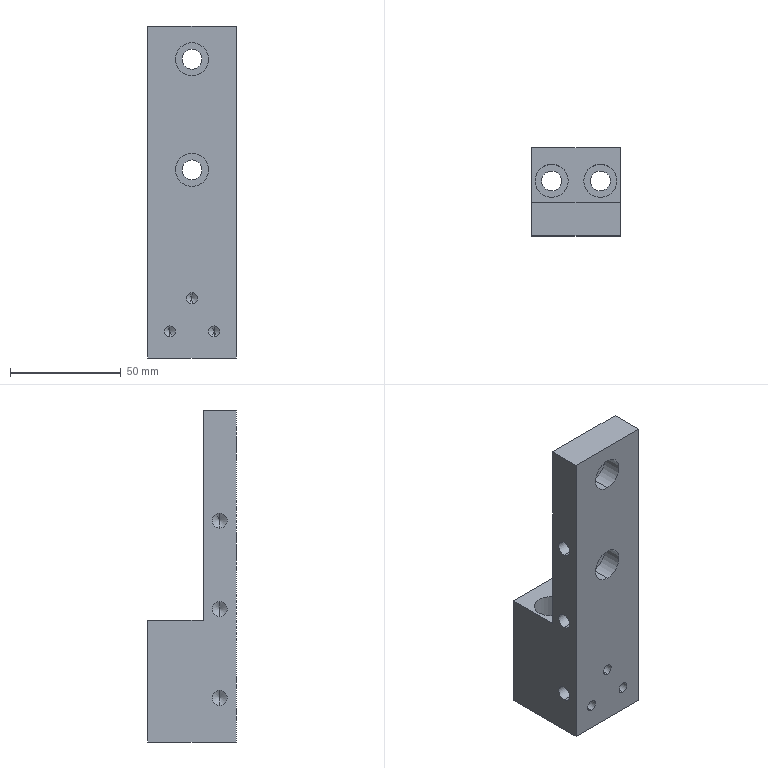Part | SolidWorks | features BaseBody 1 | 1 solid | 52 faces | box 40 x 40 x 150 mm | volume 126005 mm3 | cylinder 28 | cone 12 | plane 12 | commonest cylinder face diameters 9 x8 15 x8 5 x6 6.8 x6
STEP:
#1=CARTESIAN_POINT('',(10.,17.,-60.5));
#2=VERTEX_POINT('',#1);
#3=CARTESIAN_POINT('',(10.,17.,-65.5));
#4=VERTEX_POINT('',#3);
#5=CARTESIAN_POINT('',(10.,17.,-63.));
#6=DIRECTION('',(0.,-1.,0.));
#7=DIRECTION('',(0.,0.,-1.));
#8=AXIS2_PLACEMENT_3D('',#5,#6,#7);
#9=CIRCLE('',#8,2.5);
#10=EDGE_CURVE('',#2,#4,#9,.T.);
#11=ORIENTED_EDGE('',*,*,#10,.F.);
#12=CARTESIAN_POINT('',(10.,0.,-60.5));
#13=VERTEX_POINT('',#12);
#14=CARTESIAN_POINT('',(10.,0.,-60.5));
#15=DIRECTION('',(0.,-1.,0.));
#16=VECTOR('',#15,1000.);
#17=LINE('',#14,#16);
#18=EDGE_CURVE('',#2,#13,#17,.T.);
#19=ORIENTED_EDGE('',*,*,#18,.T.);
#20=CARTESIAN_POINT('',(10.,0.,-65.5));
#21=VERTEX_POINT('',#20);
#22=CARTESIAN_POINT('',(10.,0.,-63.));
#23=DIRECTION('',(0.,-1.,0.));
#24=DIRECTION('',(0.,0.,-1.));
#25=AXIS2_PLACEMENT_3D('',#22,#23,#24);
#26=CIRCLE('',#25,2.5);
#27=EDGE_CURVE('',#13,#21,#26,.T.);
#28=ORIENTED_EDGE('',*,*,#27,.T.);
#29=CARTESIAN_POINT('',(10.,0.,-65.5));
#30=DIRECTION('',(0.,-1.,0.));
#31=VECTOR('',#30,1000.);
#32=LINE('',#29,#31);
#33=EDGE_CURVE('',#4,#21,#32,.T.);
#34=ORIENTED_EDGE('',*,*,#33,.F.);
#35=EDGE_LOOP('',(#11,#19,#28,#34));
#36=FACE_OUTER_BOUND('',#35,.T.);
#37=CARTESIAN_POINT('',(10.,0.,-63.));
#38=DIRECTION('',(0.,-1.,0.));
#39=DIRECTION('',(0.,0.,-1.));
#40=AXIS2_PLACEMENT_3D('',#37,#38,#39);
#41=CYLINDRICAL_SURFACE('',#40,2.5);
#42=ADVANCED_FACE('',(#36),#41,.F.);
#43=CARTESIAN_POINT('',(10.,18.502,-63.));
#44=VERTEX_POINT('',#43);
#45=CARTESIAN_POINT('',(10.,17.,-65.5));
#46=DIRECTION('',(0.,-0.515,-0.8572));
#47=VECTOR('',#46,1000.);
#48=LINE('',#45,#47);
#49=EDGE_CURVE('',#44,#4,#48,.T.);
#50=ORIENTED_EDGE('',*,*,#49,.F.);
#51=CARTESIAN_POINT('',(10.,17.,-60.5));
#52=DIRECTION('',(0.,-0.515,0.8572));
#53=VECTOR('',#52,1000.);
#54=LINE('',#51,#53);
#55=EDGE_CURVE('',#44,#2,#54,.T.);
#56=ORIENTED_EDGE('',*,*,#55,.T.);
#57=ORIENTED_EDGE('',*,*,#10,.T.);
#58=EDGE_LOOP('',(#50,#56,#57));
#59=FACE_OUTER_BOUND('',#58,.T.);
#60=CARTESIAN_POINT('',(10.,17.,-63.));
#61=DIRECTION('',(0.,-1.,0.));
#62=DIRECTION('',(0.,0.,-1.));
#63=AXIS2_PLACEMENT_3D('',#60,#61,#62);
#64=CONICAL_SURFACE('',#63,2.5,1.03);
#65=ADVANCED_FACE('',(#59),#64,.F.);
#66=CARTESIAN_POINT('',(-10.,17.,-60.5));
#67=VERTEX_POINT('',#66);
#68=CARTESIAN_POINT('',(-10.,17.,-65.5));
#69=VERTEX_POINT('',#68);
#70=CARTESIAN_POINT('',(-10.,17.,-63.));
#71=DIRECTION('',(0.,-1.,0.));
#72=DIRECTION('',(0.,0.,-1.));
#73=AXIS2_PLACEMENT_3D('',#70,#71,#72);
#74=CIRCLE('',#73,2.5);
#75=EDGE_CURVE('',#67,#69,#74,.T.);
#76=ORIENTED_EDGE('',*,*,#75,.F.);
#77=CARTESIAN_POINT('',(-10.,0.,-60.5));
#78=VERTEX_POINT('',#77);
#79=CARTESIAN_POINT('',(-10.,0.,-60.5));
#80=DIRECTION('',(0.,-1.,0.));
#81=VECTOR('',#80,1000.);
#82=LINE('',#79,#81);
#83=EDGE_CURVE('',#67,#78,#82,.T.);
#84=ORIENTED_EDGE('',*,*,#83,.T.);
#85=CARTESIAN_POINT('',(-10.,0.,-65.5));
#86=VERTEX_POINT('',#85);
#87=CARTESIAN_POINT('',(-10.,0.,-63.));
#88=DIRECTION('',(0.,-1.,0.));
#89=DIRECTION('',(0.,0.,-1.));
#90=AXIS2_PLACEMENT_3D('',#87,#88,#89);
#91=CIRCLE('',#90,2.5);
#92=EDGE_CURVE('',#78,#86,#91,.T.);
#93=ORIENTED_EDGE('',*,*,#92,.T.);
#94=CARTESIAN_POINT('',(-10.,0.,-65.5));
#95=DIRECTION('',(0.,-1.,0.));
#96=VECTOR('',#95,1000.);
#97=LINE('',#94,#96);
#98=EDGE_CURVE('',#69,#86,#97,.T.);
#99=ORIENTED_EDGE('',*,*,#98,.F.);
#100=EDGE_LOOP('',(#76,#84,#93,#99));
#101=FACE_OUTER_BOUND('',#100,.T.);
#102=CARTESIAN_POINT('',(-10.,0.,-63.));
#103=DIRECTION('',(0.,-1.,0.));
#104=DIRECTION('',(0.,0.,-1.));
#105=AXIS2_PLACEMENT_3D('',#102,#103,#104);
#106=CYLINDRICAL_SURFACE('',#105,2.5);
#107=ADVANCED_FACE('',(#101),#106,.F.);
#108=CARTESIAN_POINT('',(-10.,18.502,-63.));
#109=VERTEX_POINT('',#108);
#110=CARTESIAN_POINT('',(-10.,17.,-65.5));
#111=DIRECTION('',(0.,-0.515,-0.8572));
#112=VECTOR('',#111,1000.);
#113=LINE('',#110,#112);
#114=EDGE_CURVE('',#109,#69,#113,.T.);
#115=ORIENTED_EDGE('',*,*,#114,.F.);
#116=CARTESIAN_POINT('',(-10.,17.,-60.5));
#117=DIRECTION('',(0.,-0.515,0.8572));
#118=VECTOR('',#117,1000.);
#119=LINE('',#116,#118);
#120=EDGE_CURVE('',#109,#67,#119,.T.);
#121=ORIENTED_EDGE('',*,*,#120,.T.);
#122=ORIENTED_EDGE('',*,*,#75,.T.);
#123=EDGE_LOOP('',(#115,#121,#122));
#124=FACE_OUTER_BOUND('',#123,.T.);
#125=CARTESIAN_POINT('',(-10.,17.,-63.));
#126=DIRECTION('',(0.,-1.,0.));
#127=DIRECTION('',(0.,0.,-1.));
#128=AXIS2_PLACEMENT_3D('',#125,#126,#127);
#129=CONICAL_SURFACE('',#128,2.5,1.03);
#130=ADVANCED_FACE('',(#124),#129,.F.);
#131=CARTESIAN_POINT('',(0.,17.,-45.5));
#132=VERTEX_POINT('',#131);
#133=CARTESIAN_POINT('',(0.,17.,-50.5));
#134=VERTEX_POINT('',#133);
#135=CARTESIAN_POINT('',(0.,17.,-48.));
#136=DIRECTION('',(0.,-1.,0.));
#137=DIRECTION('',(0.,0.,-1.));
#138=AXIS2_PLACEMENT_3D('',#135,#136,#137);
#139=CIRCLE('',#138,2.5);
#140=EDGE_CURVE('',#132,#134,#139,.T.);
#141=ORIENTED_EDGE('',*,*,#140,.F.);
#142=CARTESIAN_POINT('',(0.,0.,-45.5));
#143=VERTEX_POINT('',#142);
#144=CARTESIAN_POINT('',(0.,0.,-45.5));
#145=DIRECTION('',(0.,-1.,0.));
#146=VECTOR('',#145,1000.);
#147=LINE('',#144,#146);
#148=EDGE_CURVE('',#132,#143,#147,.T.);
#149=ORIENTED_EDGE('',*,*,#148,.T.);
#150=CARTESIAN_POINT('',(0.,0.,-50.5));
#151=VERTEX_POINT('',#150);
#152=CARTESIAN_POINT('',(0.,0.,-48.));
#153=DIRECTION('',(0.,-1.,0.));
#154=DIRECTION('',(0.,0.,-1.));
#155=AXIS2_PLACEMENT_3D('',#152,#153,#154);
#156=CIRCLE('',#155,2.5);
#157=EDGE_CURVE('',#143,#151,#156,.T.);
#158=ORIENTED_EDGE('',*,*,#157,.T.);
#159=CARTESIAN_POINT('',(0.,0.,-50.5));
#160=DIRECTION('',(0.,-1.,0.));
#161=VECTOR('',#160,1000.);
#162=LINE('',#159,#161);
#163=EDGE_CURVE('',#134,#151,#162,.T.);
#164=ORIENTED_EDGE('',*,*,#163,.F.);
#165=EDGE_LOOP('',(#141,#149,#158,#164));
#166=FACE_OUTER_BOUND('',#165,.T.);
#167=CARTESIAN_POINT('',(0.,0.,-48.));
#168=DIRECTION('',(0.,-1.,0.));
#169=DIRECTION('',(0.,0.,-1.));
#170=AXIS2_PLACEMENT_3D('',#167,#168,#169);
#171=CYLINDRICAL_SURFACE('',#170,2.5);
#172=ADVANCED_FACE('',(#166),#171,.F.);
#173=CARTESIAN_POINT('',(0.,18.502,-48.));
#174=VERTEX_POINT('',#173);
#175=CARTESIAN_POINT('',(0.,17.,-50.5));
#176=DIRECTION('',(0.,-0.515,-0.8572));
#177=VECTOR('',#176,1000.);
#178=LINE('',#175,#177);
#179=EDGE_CURVE('',#174,#134,#178,.T.);
#180=ORIENTED_EDGE('',*,*,#179,.F.);
#181=CARTESIAN_POINT('',(0.,17.,-45.5));
#182=DIRECTION('',(0.,-0.515,0.8572));
#183=VECTOR('',#182,1000.);
#184=LINE('',#181,#183);
#185=EDGE_CURVE('',#174,#132,#184,.T.);
#186=ORIENTED_EDGE('',*,*,#185,.T.);
#187=ORIENTED_EDGE('',*,*,#140,.T.);
#188=EDGE_LOOP('',(#180,#186,#187));
#189=FACE_OUTER_BOUND('',#188,.T.);
#190=CARTESIAN_POINT('',(0.,17.,-48.));
#191=DIRECTION('',(0.,-1.,0.));
#192=DIRECTION('',(0.,0.,-1.));
#193=AXIS2_PLACEMENT_3D('',#190,#191,#192);
#194=CONICAL_SURFACE('',#193,2.5,1.03);
#195=ADVANCED_FACE('',(#189),#194,.F.);
#196=CARTESIAN_POINT('',(2.25,7.5,-58.4));
#197=VERTEX_POINT('',#196);
#198=CARTESIAN_POINT('',(2.25,7.5,-51.6));
#199=VERTEX_POINT('',#198);
#200=CARTESIAN_POINT('',(2.25,7.5,-55.));
#201=DIRECTION('',(-1.,0.,0.));
#202=DIRECTION('',(0.,0.,1.));
#203=AXIS2_PLACEMENT_3D('',#200,#201,#202);
#204=CIRCLE('',#203,3.4);
#205=EDGE_CURVE('',#197,#199,#204,.T.);
#206=ORIENTED_EDGE('',*,*,#205,.F.);
#207=CARTESIAN_POINT('',(-20.,7.5,-58.4));
#208=VERTEX_POINT('',#207);
#209=CARTESIAN_POINT('',(-20.,7.5,-58.4));
#210=DIRECTION('',(-1.,0.,0.));
#211=VECTOR('',#210,1000.);
#212=LINE('',#209,#211);
#213=EDGE_CURVE('',#197,#208,#212,.T.);
#214=ORIENTED_EDGE('',*,*,#213,.T.);
#215=CARTESIAN_POINT('',(-20.,7.5,-51.6));
#216=VERTEX_POINT('',#215);
#217=CARTESIAN_POINT('',(-20.,7.5,-55.));
#218=DIRECTION('',(-1.,0.,0.));
#219=DIRECTION('',(0.,0.,1.));
#220=AXIS2_PLACEMENT_3D('',#217,#218,#219);
#221=CIRCLE('',#220,3.4);
#222=EDGE_CURVE('',#208,#216,#221,.T.);
#223=ORIENTED_EDGE('',*,*,#222,.T.);
#224=CARTESIAN_POINT('',(-20.,7.5,-51.6));
#225=DIRECTION('',(-1.,0.,0.));
#226=VECTOR('',#225,1000.);
#227=LINE('',#224,#226);
#228=EDGE_CURVE('',#199,#216,#227,.T.);
#229=ORIENTED_EDGE('',*,*,#228,.F.);
#230=EDGE_LOOP('',(#206,#214,#223,#229));
#231=FACE_OUTER_BOUND('',#230,.T.);
#232=CARTESIAN_POINT('',(-20.,7.5,-55.));
#233=DIRECTION('',(-1.,0.,0.));
#234=DIRECTION('',(0.,0.,1.));
#235=AXIS2_PLACEMENT_3D('',#232,#233,#234);
#236=CYLINDRICAL_SURFACE('',#235,3.4);
#237=ADVANCED_FACE('',(#231),#236,.F.);
#238=CARTESIAN_POINT('',(4.293,7.5,-55.));
#239=VERTEX_POINT('',#238);
#240=CARTESIAN_POINT('',(2.25,7.5,-51.6));
#241=DIRECTION('',(-0.515,0.,0.8572));
#242=VECTOR('',#241,1000.);
#243=LINE('',#240,#242);
#244=EDGE_CURVE('',#239,#199,#243,.T.);
#245=ORIENTED_EDGE('',*,*,#244,.F.);
#246=CARTESIAN_POINT('',(2.25,7.5,-58.4));
#247=DIRECTION('',(-0.515,0.,-0.8572));
#248=VECTOR('',#247,1000.);
#249=LINE('',#246,#248);
#250=EDGE_CURVE('',#239,#197,#249,.T.);
#251=ORIENTED_EDGE('',*,*,#250,.T.);
#252=ORIENTED_EDGE('',*,*,#205,.T.);
#253=EDGE_LOOP('',(#245,#251,#252));
#254=FACE_OUTER_BOUND('',#253,.T.);
#255=CARTESIAN_POINT('',(2.25,7.5,-55.));
#256=DIRECTION('',(-1.,0.,0.));
#257=DIRECTION('',(0.,0.,1.));
#258=AXIS2_PLACEMENT_3D('',#255,#256,#257);
#259=CONICAL_SURFACE('',#258,3.4,1.03);
#260=ADVANCED_FACE('',(#254),#259,.F.);
#261=CARTESIAN_POINT('',(2.25,7.5,-18.4));
#262=VERTEX_POINT('',#261);
#263=CARTESIAN_POINT('',(2.25,7.5,-11.6));
#264=VERTEX_POINT('',#263);
#265=CARTESIAN_POINT('',(2.25,7.5,-15.));
#266=DIRECTION('',(-1.,0.,0.));
#267=DIRECTION('',(0.,0.,1.));
#268=AXIS2_PLACEMENT_3D('',#265,#266,#267);
#269=CIRCLE('',#268,3.4);
#270=EDGE_CURVE('',#262,#264,#269,.T.);
#271=ORIENTED_EDGE('',*,*,#270,.F.);
#272=CARTESIAN_POINT('',(-20.,7.5,-18.4));
#273=VERTEX_POINT('',#272);
#274=CARTESIAN_POINT('',(-20.,7.5,-18.4));
#275=DIRECTION('',(-1.,0.,0.));
#276=VECTOR('',#275,1000.);
#277=LINE('',#274,#276);
#278=EDGE_CURVE('',#262,#273,#277,.T.);
#279=ORIENTED_EDGE('',*,*,#278,.T.);
#280=CARTESIAN_POINT('',(-20.,7.5,-11.6));
#281=VERTEX_POINT('',#280);
#282=CARTESIAN_POINT('',(-20.,7.5,-15.));
#283=DIRECTION('',(-1.,0.,0.));
#284=DIRECTION('',(0.,0.,1.));
#285=AXIS2_PLACEMENT_3D('',#282,#283,#284);
#286=CIRCLE('',#285,3.4);
#287=EDGE_CURVE('',#273,#281,#286,.T.);
#288=ORIENTED_EDGE('',*,*,#287,.T.);
#289=CARTESIAN_POINT('',(-20.,7.5,-11.6));
#290=DIRECTION('',(-1.,0.,0.));
#291=VECTOR('',#290,1000.);
#292=LINE('',#289,#291);
#293=EDGE_CURVE('',#264,#281,#292,.T.);
#294=ORIENTED_EDGE('',*,*,#293,.F.);
#295=EDGE_LOOP('',(#271,#279,#288,#294));
#296=FACE_OUTER_BOUND('',#295,.T.);
#297=CARTESIAN_POINT('',(-20.,7.5,-15.));
#298=DIRECTION('',(-1.,0.,0.));
#299=DIRECTION('',(0.,0.,1.));
#300=AXIS2_PLACEMENT_3D('',#297,#298,#299);
#301=CYLINDRICAL_SURFACE('',#300,3.4);
#302=ADVANCED_FACE('',(#296),#301,.F.);
#303=CARTESIAN_POINT('',(4.293,7.5,-15.));
#304=VERTEX_POINT('',#303);
#305=CARTESIAN_POINT('',(2.25,7.5,-11.6));
#306=DIRECTION('',(-0.515,0.,0.8572));
#307=VECTOR('',#306,1000.);
#308=LINE('',#305,#307);
#309=EDGE_CURVE('',#304,#264,#308,.T.);
#310=ORIENTED_EDGE('',*,*,#309,.F.);
#311=CARTESIAN_POINT('',(2.25,7.5,-18.4));
#312=DIRECTION('',(-0.515,0.,-0.8572));
#313=VECTOR('',#312,1000.);
#314=LINE('',#311,#313);
#315=EDGE_CURVE('',#304,#262,#314,.T.);
#316=ORIENTED_EDGE('',*,*,#315,.T.);
#317=ORIENTED_EDGE('',*,*,#270,.T.);
#318=EDGE_LOOP('',(#310,#316,#317));
#319=FACE_OUTER_BOUND('',#318,.T.);
#320=CARTESIAN_POINT('',(2.25,7.5,-15.));
#321=DIRECTION('',(-1.,0.,0.));
#322=DIRECTION('',(0.,0.,1.));
#323=AXIS2_PLACEMENT_3D('',#320,#321,#322);
#324=CONICAL_SURFACE('',#323,3.4,1.03);
#325=ADVANCED_FACE('',(#319),#324,.F.);
#326=CARTESIAN_POINT('',(2.25,7.5,21.6));
#327=VERTEX_POINT('',#326);
#328=CARTESIAN_POINT('',(2.25,7.5,28.4));
#329=VERTEX_POINT('',#328);
#330=CARTESIAN_POINT('',(2.25,7.5,25.));
#331=DIRECTION('',(-1.,0.,0.));
#332=DIRECTION('',(0.,0.,1.));
#333=AXIS2_PLACEMENT_3D('',#330,#331,#332);
#334=CIRCLE('',#333,3.4);
#335=EDGE_CURVE('',#327,#329,#334,.T.);
#336=ORIENTED_EDGE('',*,*,#335,.F.);
#337=CARTESIAN_POINT('',(-20.,7.5,21.6));
#338=VERTEX_POINT('',#337);
#339=CARTESIAN_POINT('',(-20.,7.5,21.6));
#340=DIRECTION('',(-1.,0.,0.));
#341=VECTOR('',#340,1000.);
#342=LINE('',#339,#341);
#343=EDGE_CURVE('',#327,#338,#342,.T.);
#344=ORIENTED_EDGE('',*,*,#343,.T.);
#345=CARTESIAN_POINT('',(-20.,7.5,28.4));
#346=VERTEX_POINT('',#345);
#347=CARTESIAN_POINT('',(-20.,7.5,25.));
#348=DIRECTION('',(-1.,0.,0.));
#349=DIRECTION('',(0.,0.,1.));
#350=AXIS2_PLACEMENT_3D('',#347,#348,#349);
#351=CIRCLE('',#350,3.4);
#352=EDGE_CURVE('',#338,#346,#351,.T.);
#353=ORIENTED_EDGE('',*,*,#352,.T.);
#354=CARTESIAN_POINT('',(-20.,7.5,28.4));
#355=DIRECTION('',(-1.,0.,0.));
#356=VECTOR('',#355,1000.);
#357=LINE('',#354,#356);
#358=EDGE_CURVE('',#329,#346,#357,.T.);
#359=ORIENTED_EDGE('',*,*,#358,.F.);
#360=EDGE_LOOP('',(#336,#344,#353,#359));
#361=FACE_OUTER_BOUND('',#360,.T.);
#362=CARTESIAN_POINT('',(-20.,7.5,25.));
#363=DIRECTION('',(-1.,0.,0.));
#364=DIRECTION('',(0.,0.,1.));
#365=AXIS2_PLACEMENT_3D('',#362,#363,#364);
#366=CYLINDRICAL_SURFACE('',#365,3.4);
#367=ADVANCED_FACE('',(#361),#366,.F.);
#368=CARTESIAN_POINT('',(4.293,7.5,25.));
#369=VERTEX_POINT('',#368);
#370=CARTESIAN_POINT('',(2.25,7.5,28.4));
#371=DIRECTION('',(-0.515,0.,0.8572));
#372=VECTOR('',#371,1000.);
#373=LINE('',#370,#372);
#374=EDGE_CURVE('',#369,#329,#373,.T.);
#375=ORIENTED_EDGE('',*,*,#374,.F.);
#376=CARTESIAN_POINT('',(2.25,7.5,21.6));
#377=DIRECTION('',(-0.515,0.,-0.8572));
#378=VECTOR('',#377,1000.);
#379=LINE('',#376,#378);
#380=EDGE_CURVE('',#369,#327,#379,.T.);
#381=ORIENTED_EDGE('',*,*,#380,.T.);
#382=ORIENTED_EDGE('',*,*,#335,.T.);
#383=EDGE_LOOP('',(#375,#381,#382));
#384=FACE_OUTER_BOUND('',#383,.T.);
#385=CARTESIAN_POINT('',(2.25,7.5,25.));
#386=DIRECTION('',(-1.,0.,0.));
#387=DIRECTION('',(0.,0.,1.));
#388=AXIS2_PLACEMENT_3D('',#385,#386,#387);
#389=CONICAL_SURFACE('',#388,3.4,1.03);
#390=ADVANCED_FACE('',(#384),#389,.F.);
#391=CARTESIAN_POINT('',(3.5,25.,-40.));
#392=VERTEX_POINT('',#391);
#393=CARTESIAN_POINT('',(18.5,25.,-40.));
#394=VERTEX_POINT('',#393);
#395=CARTESIAN_POINT('',(11.,25.,-40.));
#396=DIRECTION('',(0.,0.,1.));
#397=DIRECTION('',(1.,0.,0.));
#398=AXIS2_PLACEMENT_3D('',#395,#396,#397);
#399=CIRCLE('',#398,7.5);
#400=EDGE_CURVE('',#392,#394,#399,.T.);
#401=ORIENTED_EDGE('',*,*,#400,.F.);
#402=CARTESIAN_POINT('',(3.5,25.,-20.));
#403=VERTEX_POINT('',#402);
#404=CARTESIAN_POINT('',(3.5,25.,-20.));
#405=DIRECTION('',(0.,0.,1.));
#406=VECTOR('',#405,1000.);
#407=LINE('',#404,#406);
#408=EDGE_CURVE('',#392,#403,#407,.T.);
#409=ORIENTED_EDGE('',*,*,#408,.T.);
#410=CARTESIAN_POINT('',(18.5,25.,-20.));
#411=VERTEX_POINT('',#410);
#412=CARTESIAN_POINT('',(11.,25.,-20.));
#413=DIRECTION('',(0.,0.,1.));
#414=DIRECTION('',(1.,0.,0.));
#415=AXIS2_PLACEMENT_3D('',#412,#413,#414);
#416=CIRCLE('',#415,7.5);
#417=EDGE_CURVE('',#403,#411,#416,.T.);
#418=ORIENTED_EDGE('',*,*,#417,.T.);
#419=CARTESIAN_POINT('',(18.5,25.,-20.));
#420=DIRECTION('',(0.,0.,1.));
#421=VECTOR('',#420,1000.);
#422=LINE('',#419,#421);
#423=EDGE_CURVE('',#394,#411,#422,.T.);
#424=ORIENTED_EDGE('',*,*,#423,.F.);
#425=EDGE_LOOP('',(#401,#409,#418,#424));
#426=FACE_OUTER_BOUND('',#425,.T.);
#427=CARTESIAN_POINT('',(11.,25.,-20.));
#428=DIRECTION('',(0.,0.,1.));
#429=DIRECTION('',(1.,0.,0.));
#430=AXIS2_PLACEMENT_3D('',#427,#428,#429);
#431=CYLINDRICAL_SURFACE('',#430,7.5);
#432=ADVANCED_FACE('',(#426),#431,.F.);
#433=CARTESIAN_POINT('',(6.5,25.,-75.));
#434=VERTEX_POINT('',#433);
#435=CARTESIAN_POINT('',(15.5,25.,-75.));
#436=VERTEX_POINT('',#435);
#437=CARTESIAN_POINT('',(11.,25.,-75.));
#438=DIRECTION('',(0.,0.,1.));
#439=DIRECTION('',(1.,0.,0.));
#440=AXIS2_PLACEMENT_3D('',#437,#438,#439);
#441=CIRCLE('',#440,4.5);
#442=EDGE_CURVE('',#434,#436,#441,.T.);
#443=ORIENTED_EDGE('',*,*,#442,.F.);
#444=CARTESIAN_POINT('',(6.5,25.,-40.));
#445=VERTEX_POINT('',#444);
#446=CARTESIAN_POINT('',(6.5,25.,-20.));
#447=DIRECTION('',(0.,0.,1.));
#448=VECTOR('',#447,1000.);
#449=LINE('',#446,#448);
#450=EDGE_CURVE('',#434,#445,#449,.T.);
#451=ORIENTED_EDGE('',*,*,#450,.T.);
#452=CARTESIAN_POINT('',(15.5,25.,-40.));
#453=VERTEX_POINT('',#452);
#454=CARTESIAN_POINT('',(11.,25.,-40.));
#455=DIRECTION('',(0.,0.,1.));
#456=DIRECTION('',(1.,0.,0.));
#457=AXIS2_PLACEMENT_3D('',#454,#455,#456);
#458=CIRCLE('',#457,4.5);
#459=EDGE_CURVE('',#445,#453,#458,.T.);
#460=ORIENTED_EDGE('',*,*,#459,.T.);
#461=CARTESIAN_POINT('',(15.5,25.,-20.));
#462=DIRECTION('',(0.,0.,1.));
#463=VECTOR('',#462,1000.);
#464=LINE('',#461,#463);
#465=EDGE_CURVE('',#436,#453,#464,.T.);
#466=ORIENTED_EDGE('',*,*,#465,.F.);
#467=EDGE_LOOP('',(#443,#451,#460,#466));
#468=FACE_OUTER_BOUND('',#467,.T.);
#469=CARTESIAN_POINT('',(11.,25.,-20.));
#470=DIRECTION('',(0.,0.,1.));
#471=DIRECTION('',(1.,0.,0.));
#472=AXIS2_PLACEMENT_3D('',#469,#470,#471);
#473=CYLINDRICAL_SURFACE('',#472,4.5);
#474=ADVANCED_FACE('',(#468),#473,.F.);
#475=CARTESIAN_POINT('',(-18.5,25.,-40.));
#476=VERTEX_POINT('',#475);
#477=CARTESIAN_POINT('',(-3.5,25.,-40.));
#478=VERTEX_POINT('',#477);
#479=CARTESIAN_POINT('',(-11.,25.,-40.));
#480=DIRECTION('',(0.,0.,1.));
#481=DIRECTION('',(1.,0.,0.));
#482=AXIS2_PLACEMENT_3D('',#479,#480,#481);
#483=CIRCLE('',#482,7.5);
#484=EDGE_CURVE('',#476,#478,#483,.T.);
#485=ORIENTED_EDGE('',*,*,#484,.F.);
#486=CARTESIAN_POINT('',(-18.5,25.,-20.));
#487=VERTEX_POINT('',#486);
#488=CARTESIAN_POINT('',(-18.5,25.,-20.));
#489=DIRECTION('',(0.,0.,1.));
#490=VECTOR('',#489,1000.);
#491=LINE('',#488,#490);
#492=EDGE_CURVE('',#476,#487,#491,.T.);
#493=ORIENTED_EDGE('',*,*,#492,.T.);
#494=CARTESIAN_POINT('',(-3.5,25.,-20.));
#495=VERTEX_POINT('',#494);
#496=CARTESIAN_POINT('',(-11.,25.,-20.));
#497=DIRECTION('',(0.,0.,1.));
#498=DIRECTION('',(1.,0.,0.));
#499=AXIS2_PLACEMENT_3D('',#496,#497,#498);
#500=CIRCLE('',#499,7.5);
#501=EDGE_CURVE('',#487,#495,#500,.T.);
#502=ORIENTED_EDGE('',*,*,#501,.T.);
#503=CARTESIAN_POINT('',(-3.5,25.,-20.));
#504=DIRECTION('',(0.,0.,1.));
#505=VECTOR('',#504,1000.);
#506=LINE('',#503,#505);
#507=EDGE_CURVE('',#478,#495,#506,.T.);
#508=ORIENTED_EDGE('',*,*,#507,.F.);
#509=EDGE_LOOP('',(#485,#493,#502,#508));
#510=FACE_OUTER_BOUND('',#509,.T.);
#511=CARTESIAN_POINT('',(-11.,25.,-20.));
#512=DIRECTION('',(0.,0.,1.));
#513=DIRECTION('',(1.,0.,0.));
#514=AXIS2_PLACEMENT_3D('',#511,#512,#513);
#515=CYLINDRICAL_SURFACE('',#514,7.5);
#516=ADVANCED_FACE('',(#510),#515,.F.);
#517=CARTESIAN_POINT('',(-15.5,25.,-75.));
#518=VERTEX_POINT('',#517);
#519=CARTESIAN_POINT('',(-6.5,25.,-75.));
#520=VERTEX_POINT('',#519);
#521=CARTESIAN_POINT('',(-11.,25.,-75.));
#522=DIRECTION('',(0.,0.,1.));
#523=DIRECTION('',(1.,0.,0.));
#524=AXIS2_PLACEMENT_3D('',#521,#522,#523);
#525=CIRCLE('',#524,4.5);
#526=EDGE_CURVE('',#518,#520,#525,.T.);
#527=ORIENTED_EDGE('',*,*,#526,.F.);
#528=CARTESIAN_POINT('',(-15.5,25.,-40.));
#529=VERTEX_POINT('',#528);
#530=CARTESIAN_POINT('',(-15.5,25.,-20.));
#531=DIRECTION('',(0.,0.,1.));
#532=VECTOR('',#531,1000.);
#533=LINE('',#530,#532);
#534=EDGE_CURVE('',#518,#529,#533,.T.);
#535=ORIENTED_EDGE('',*,*,#534,.T.);
#536=CARTESIAN_POINT('',(-6.5,25.,-40.));
#537=VERTEX_POINT('',#536);
#538=CARTESIAN_POINT('',(-11.,25.,-40.));
#539=DIRECTION('',(0.,0.,1.));
#540=DIRECTION('',(1.,0.,0.));
#541=AXIS2_PLACEMENT_3D('',#538,#539,#540);
#542=CIRCLE('',#541,4.5);
#543=EDGE_CURVE('',#529,#537,#542,.T.);
#544=ORIENTED_EDGE('',*,*,#543,.T.);
#545=CARTESIAN_POINT('',(-6.5,25.,-20.));
#546=DIRECTION('',(0.,0.,1.));
#547=VECTOR('',#546,1000.);
#548=LINE('',#545,#547);
#549=EDGE_CURVE('',#520,#537,#548,.T.);
#550=ORIENTED_EDGE('',*,*,#549,.F.);
#551=EDGE_LOOP('',(#527,#535,#544,#550));
#552=FACE_OUTER_BOUND('',#551,.T.);
#553=CARTESIAN_POINT('',(-11.,25.,-20.));
#554=DIRECTION('',(0.,0.,1.));
#555=DIRECTION('',(1.,0.,0.));
#556=AXIS2_PLACEMENT_3D('',#553,#554,#555);
#557=CYLINDRICAL_SURFACE('',#556,4.5);
#558=ADVANCED_FACE('',(#552),#557,.F.);
#559=CARTESIAN_POINT('',(0.,9.,67.5));
#560=VERTEX_POINT('',#559);
#561=CARTESIAN_POINT('',(0.,9.,52.5));
#562=VERTEX_POINT('',#561);
#563=CARTESIAN_POINT('',(0.,9.,60.));
#564=DIRECTION('',(0.,-1.,0.));
#565=DIRECTION('',(0.,0.,-1.));
#566=AXIS2_PLACEMENT_3D('',#563,#564,#565);
#567=CIRCLE('',#566,7.5);
#568=EDGE_CURVE('',#560,#562,#567,.T.);
#569=ORIENTED_EDGE('',*,*,#568,.F.);
#570=CARTESIAN_POINT('',(0.,0.,67.5));
#571=VERTEX_POINT('',#570);
#572=CARTESIAN_POINT('',(0.,0.,67.5));
#573=DIRECTION('',(0.,-1.,0.));
#574=VECTOR('',#573,1000.);
#575=LINE('',#572,#574);
#576=EDGE_CURVE('',#560,#571,#575,.T.);
#577=ORIENTED_EDGE('',*,*,#576,.T.);
#578=CARTESIAN_POINT('',(0.,0.,52.5));
#579=VERTEX_POINT('',#578);
#580=CARTESIAN_POINT('',(0.,0.,60.));
#581=DIRECTION('',(0.,-1.,0.));
#582=DIRECTION('',(0.,0.,-1.));
#583=AXIS2_PLACEMENT_3D('',#580,#581,#582);
#584=CIRCLE('',#583,7.5);
#585=EDGE_CURVE('',#571,#579,#584,.T.);
#586=ORIENTED_EDGE('',*,*,#585,.T.);
#587=CARTESIAN_POINT('',(0.,0.,52.5));
#588=DIRECTION('',(0.,-1.,0.));
#589=VECTOR('',#588,1000.);
#590=LINE('',#587,#589);
#591=EDGE_CURVE('',#562,#579,#590,.T.);
#592=ORIENTED_EDGE('',*,*,#591,.F.);
#593=EDGE_LOOP('',(#569,#577,#586,#592));
#594=FACE_OUTER_BOUND('',#593,.T.);
#595=CARTESIAN_POINT('',(0.,0.,60.));
#596=DIRECTION('',(0.,-1.,0.));
#597=DIRECTION('',(0.,0.,-1.));
#598=AXIS2_PLACEMENT_3D('',#595,#596,#597);
#599=CYLINDRICAL_SURFACE('',#598,7.5);
#600=ADVANCED_FACE('',(#594),#599,.F.);
#601=CARTESIAN_POINT('',(0.,15.,64.5));
#602=VERTEX_POINT('',#601);
#603=CARTESIAN_POINT('',(0.,15.,55.5));
#604=VERTEX_POINT('',#603);
#605=CARTESIAN_POINT('',(0.,15.,60.));
#606=DIRECTION('',(0.,-1.,0.));
#607=DIRECTION('',(0.,0.,-1.));
#608=AXIS2_PLACEMENT_3D('',#605,#606,#607);
#609=CIRCLE('',#608,4.5);
#610=EDGE_CURVE('',#602,#604,#609,.T.);
#611=ORIENTED_EDGE('',*,*,#610,.F.);
#612=CARTESIAN_POINT('',(0.,9.,64.5));
#613=VERTEX_POINT('',#612);
#614=CARTESIAN_POINT('',(0.,0.,64.5));
#615=DIRECTION('',(0.,-1.,0.));
#616=VECTOR('',#615,1000.);
#617=LINE('',#614,#616);
#618=EDGE_CURVE('',#602,#613,#617,.T.);
#619=ORIENTED_EDGE('',*,*,#618,.T.);
#620=CARTESIAN_POINT('',(0.,9.,55.5));
#621=VERTEX_POINT('',#620);
#622=CARTESIAN_POINT('',(0.,9.,60.));
#623=DIRECTION('',(0.,-1.,0.));
#624=DIRECTION('',(0.,0.,-1.));
#625=AXIS2_PLACEMENT_3D('',#622,#623,#624);
#626=CIRCLE('',#625,4.5);
#627=EDGE_CURVE('',#613,#621,#626,.T.);
#628=ORIENTED_EDGE('',*,*,#627,.T.);
#629=CARTESIAN_POINT('',(0.,0.,55.5));
#630=DIRECTION('',(0.,-1.,0.));
#631=VECTOR('',#630,1000.);
#632=LINE('',#629,#631);
#633=EDGE_CURVE('',#604,#621,#632,.T.);
#634=ORIENTED_EDGE('',*,*,#633,.F.);
#635=EDGE_LOOP('',(#611,#619,#628,#634));
#636=FACE_OUTER_BOUND('',#635,.T.);
#637=CARTESIAN_POINT('',(0.,0.,60.));
#638=DIRECTION('',(0.,-1.,0.));
#639=DIRECTION('',(0.,0.,-1.));
#640=AXIS2_PLACEMENT_3D('',#637,#638,#639);
#641=CYLINDRICAL_SURFACE('',#640,4.5);
#642=ADVANCED_FACE('',(#636),#641,.F.);
#643=CARTESIAN_POINT('',(0.,9.,17.5));
#644=VERTEX_POINT('',#643);
#645=CARTESIAN_POINT('',(0.,9.,2.5));
#646=VERTEX_POINT('',#645);
#647=CARTESIAN_POINT('',(0.,9.,10.));
#648=DIRECTION('',(0.,-1.,0.));
#649=DIRECTION('',(0.,0.,-1.));
#650=AXIS2_PLACEMENT_3D('',#647,#648,#649);
#651=CIRCLE('',#650,7.5);
#652=EDGE_CURVE('',#644,#646,#651,.T.);
#653=ORIENTED_EDGE('',*,*,#652,.F.);
#654=CARTESIAN_POINT('',(0.,0.,17.5));
#655=VERTEX_POINT('',#654);
#656=CARTESIAN_POINT('',(0.,0.,17.5));
#657=DIRECTION('',(0.,-1.,0.));
#658=VECTOR('',#657,1000.);
#659=LINE('',#656,#658);
#660=EDGE_CURVE('',#644,#655,#659,.T.);
#661=ORIENTED_EDGE('',*,*,#660,.T.);
#662=CARTESIAN_POINT('',(0.,0.,2.5));
#663=VERTEX_POINT('',#662);
#664=CARTESIAN_POINT('',(0.,0.,10.));
#665=DIRECTION('',(0.,-1.,0.));
#666=DIRECTION('',(0.,0.,-1.));
#667=AXIS2_PLACEMENT_3D('',#664,#665,#666);
#668=CIRCLE('',#667,7.5);
#669=EDGE_CURVE('',#655,#663,#668,.T.);
#670=ORIENTED_EDGE('',*,*,#669,.T.);
#671=CARTESIAN_POINT('',(0.,0.,2.5));
#672=DIRECTION('',(0.,-1.,0.));
#673=VECTOR('',#672,1000.);
#674=LINE('',#671,#673);
#675=EDGE_CURVE('',#646,#663,#674,.T.);
#676=ORIENTED_EDGE('',*,*,#675,.F.);
#677=EDGE_LOOP('',(#653,#661,#670,#676));
#678=FACE_OUTER_BOUND('',#677,.T.);
#679=CARTESIAN_POINT('',(0.,0.,10.));
#680=DIRECTION('',(0.,-1.,0.));
#681=DIRECTION('',(0.,0.,-1.));
#682=AXIS2_PLACEMENT_3D('',#679,#680,#681);
#683=CYLINDRICAL_SURFACE('',#682,7.5);
#684=ADVANCED_FACE('',(#678),#683,.F.);
#685=CARTESIAN_POINT('',(0.,15.,14.5));
#686=VERTEX_POINT('',#685);
#687=CARTESIAN_POINT('',(0.,15.,5.5));
#688=VERTEX_POINT('',#687);
#689=CARTESIAN_POINT('',(0.,15.,10.));
#690=DIRECTION('',(0.,-1.,0.));
#691=DIRECTION('',(0.,0.,-1.));
#692=AXIS2_PLACEMENT_3D('',#689,#690,#691);
#693=CIRCLE('',#692,4.5);
#694=EDGE_CURVE('',#686,#688,#693,.T.);
#695=ORIENTED_EDGE('',*,*,#694,.F.);
#696=CARTESIAN_POINT('',(0.,9.,14.5));
#697=VERTEX_POINT('',#696);
#698=CARTESIAN_POINT('',(0.,0.,14.5));
#699=DIRECTION('',(0.,-1.,0.));
#700=VECTOR('',#699,1000.);
#701=LINE('',#698,#700);
#702=EDGE_CURVE('',#686,#697,#701,.T.);
#703=ORIENTED_EDGE('',*,*,#702,.T.);
#704=CARTESIAN_POINT('',(0.,9.,5.5));
#705=VERTEX_POINT('',#704);
#706=CARTESIAN_POINT('',(0.,9.,10.));
#707=DIRECTION('',(0.,-1.,0.));
#708=DIRECTION('',(0.,0.,-1.));
#709=AXIS2_PLACEMENT_3D('',#706,#707,#708);
#710=CIRCLE('',#709,4.5);
#711=EDGE_CURVE('',#697,#705,#710,.T.);
#712=ORIENTED_EDGE('',*,*,#711,.T.);
#713=CARTESIAN_POINT('',(0.,0.,5.5));
#714=DIRECTION('',(0.,-1.,0.));
#715=VECTOR('',#714,1000.);
#716=LINE('',#713,#715);
#717=EDGE_CURVE('',#688,#705,#716,.T.);
#718=ORIENTED_EDGE('',*,*,#717,.F.);
#719=EDGE_LOOP('',(#695,#703,#712,#718));
#720=FACE_OUTER_BOUND('',#719,.T.);
#721=CARTESIAN_POINT('',(0.,0.,10.));
#722=DIRECTION('',(0.,-1.,0.));
#723=DIRECTION('',(0.,0.,-1.));
#724=AXIS2_PLACEMENT_3D('',#721,#722,#723);
#725=CYLINDRICAL_SURFACE('',#724,4.5);
#726=ADVANCED_FACE('',(#720),#725,.F.);
#727=CARTESIAN_POINT('',(11.,25.,-40.));
#728=DIRECTION('',(0.,0.,1.));
#729=DIRECTION('',(1.,0.,0.));
#730=AXIS2_PLACEMENT_3D('',#727,#728,#729);
#731=CIRCLE('',#730,4.5);
#732=EDGE_CURVE('',#453,#445,#731,.T.);
#733=ORIENTED_EDGE('',*,*,#732,.F.);
#734=ORIENTED_EDGE('',*,*,#459,.F.);
#735=EDGE_LOOP('',(#733,#734));
#736=FACE_BOUND('',#735,.T.);
#737=CARTESIAN_POINT('',(11.,25.,-40.));
#738=DIRECTION('',(0.,0.,1.));
#739=DIRECTION('',(1.,0.,0.));
#740=AXIS2_PLACEMENT_3D('',#737,#738,#739);
#741=CIRCLE('',#740,7.5);
#742=EDGE_CURVE('',#394,#392,#741,.T.);
#743=ORIENTED_EDGE('',*,*,#742,.T.);
#744=ORIENTED_EDGE('',*,*,#400,.T.);
#745=EDGE_LOOP('',(#743,#744));
#746=FACE_OUTER_BOUND('',#745,.T.);
#747=CARTESIAN_POINT('',(15.5,25.,-40.));
#748=DIRECTION('',(0.,0.,-1.));
#749=DIRECTION('',(0.,-1.,0.));
#750=AXIS2_PLACEMENT_3D('',#747,#748,#749);
#751=PLANE('',#750);
#752=ADVANCED_FACE('',(#736,#746),#751,.F.);
#753=CARTESIAN_POINT('',(-11.,25.,-40.));
#754=DIRECTION('',(0.,0.,1.));
#755=DIRECTION('',(1.,0.,0.));
#756=AXIS2_PLACEMENT_3D('',#753,#754,#755);
#757=CIRCLE('',#756,4.5);
#758=EDGE_CURVE('',#537,#529,#757,.T.);
#759=ORIENTED_EDGE('',*,*,#758,.F.);
#760=ORIENTED_EDGE('',*,*,#543,.F.);
#761=EDGE_LOOP('',(#759,#760));
#762=FACE_BOUND('',#761,.T.);
#763=CARTESIAN_POINT('',(-11.,25.,-40.));
#764=DIRECTION('',(0.,0.,1.));
#765=DIRECTION('',(1.,0.,0.));
#766=AXIS2_PLACEMENT_3D('',#763,#764,#765);
#767=CIRCLE('',#766,7.5);
#768=EDGE_CURVE('',#478,#476,#767,.T.);
#769=ORIENTED_EDGE('',*,*,#768,.T.);
#770=ORIENTED_EDGE('',*,*,#484,.T.);
#771=EDGE_LOOP('',(#769,#770));
#772=FACE_OUTER_BOUND('',#771,.T.);
#773=CARTESIAN_POINT('',(-6.5,25.,-40.));
#774=DIRECTION('',(0.,0.,-1.));
#775=DIRECTION('',(0.,-1.,0.));
#776=AXIS2_PLACEMENT_3D('',#773,#774,#775);
#777=PLANE('',#776);
#778=ADVANCED_FACE('',(#762,#772),#777,.F.);
#779=CARTESIAN_POINT('',(0.,9.,60.));
#780=DIRECTION('',(0.,-1.,0.));
#781=DIRECTION('',(0.,0.,-1.));
#782=AXIS2_PLACEMENT_3D('',#779,#780,#781);
#783=CIRCLE('',#782,4.5);
#784=EDGE_CURVE('',#621,#613,#783,.T.);
#785=ORIENTED_EDGE('',*,*,#784,.F.);
#786=ORIENTED_EDGE('',*,*,#627,.F.);
#787=EDGE_LOOP('',(#785,#786));
#788=FACE_BOUND('',#787,.T.);
#789=CARTESIAN_POINT('',(0.,9.,60.));
#790=DIRECTION('',(0.,-1.,0.));
#791=DIRECTION('',(0.,0.,-1.));
#792=AXIS2_PLACEMENT_3D('',#789,#790,#791);
#793=CIRCLE('',#792,7.5);
#794=EDGE_CURVE('',#562,#560,#793,.T.);
#795=ORIENTED_EDGE('',*,*,#794,.T.);
#796=ORIENTED_EDGE('',*,*,#568,.T.);
#797=EDGE_LOOP('',(#795,#796));
#798=FACE_OUTER_BOUND('',#797,.T.);
#799=CARTESIAN_POINT('',(4.5,9.,60.));
#800=DIRECTION('',(0.,1.,0.));
#801=DIRECTION('',(1.,0.,0.));
#802=AXIS2_PLACEMENT_3D('',#799,#800,#801);
#803=PLANE('',#802);
#804=ADVANCED_FACE('',(#788,#798),#803,.F.);
#805=CARTESIAN_POINT('',(0.,9.,10.));
#806=DIRECTION('',(0.,-1.,0.));
#807=DIRECTION('',(0.,0.,-1.));
#808=AXIS2_PLACEMENT_3D('',#805,#806,#807);
#809=CIRCLE('',#808,4.5);
#810=EDGE_CURVE('',#705,#697,#809,.T.);
#811=ORIENTED_EDGE('',*,*,#810,.F.);
#812=ORIENTED_EDGE('',*,*,#711,.F.);
#813=EDGE_LOOP('',(#811,#812));
#814=FACE_BOUND('',#813,.T.);
#815=CARTESIAN_POINT('',(0.,9.,10.));
#816=DIRECTION('',(0.,-1.,0.));
#817=DIRECTION('',(0.,0.,-1.));
#818=AXIS2_PLACEMENT_3D('',#815,#816,#817);
#819=CIRCLE('',#818,7.5);
#820=EDGE_CURVE('',#646,#644,#819,.T.);
#821=ORIENTED_EDGE('',*,*,#820,.T.);
#822=ORIENTED_EDGE('',*,*,#652,.T.);
#823=EDGE_LOOP('',(#821,#822));
#824=FACE_OUTER_BOUND('',#823,.T.);
#825=CARTESIAN_POINT('',(4.5,9.,10.));
#826=DIRECTION('',(0.,1.,0.));
#827=DIRECTION('',(1.,0.,0.));
#828=AXIS2_PLACEMENT_3D('',#825,#826,#827);
#829=PLANE('',#828);
#830=ADVANCED_FACE('',(#814,#824),#829,.F.);
#831=CARTESIAN_POINT('',(0.,15.,10.));
#832=DIRECTION('',(0.,-1.,0.));
#833=DIRECTION('',(0.,0.,-1.));
#834=AXIS2_PLACEMENT_3D('',#831,#832,#833);
#835=CIRCLE('',#834,4.5);
#836=EDGE_CURVE('',#688,#686,#835,.T.);
#837=ORIENTED_EDGE('',*,*,#836,.T.);
#838=ORIENTED_EDGE('',*,*,#694,.T.);
#839=EDGE_LOOP('',(#837,#838));
#840=FACE_BOUND('',#839,.T.);
#841=CARTESIAN_POINT('',(0.,15.,60.));
#842=DIRECTION('',(0.,-1.,0.));
#843=DIRECTION('',(0.,0.,-1.));
#844=AXIS2_PLACEMENT_3D('',#841,#842,#843);
#845=CIRCLE('',#844,4.5);
#846=EDGE_CURVE('',#604,#602,#845,.T.);
#847=ORIENTED_EDGE('',*,*,#846,.T.);
#848=ORIENTED_EDGE('',*,*,#610,.T.);
#849=EDGE_LOOP('',(#847,#848));
#850=FACE_BOUND('',#849,.T.);
#851=CARTESIAN_POINT('',(-20.,15.,-20.));
#852=VERTEX_POINT('',#851);
#853=CARTESIAN_POINT('',(-20.,15.,75.));
#854=VERTEX_POINT('',#853);
#855=CARTESIAN_POINT('',(-20.,15.,75.));
#856=DIRECTION('',(0.,0.,1.));
#857=VECTOR('',#856,1000.);
#858=LINE('',#855,#857);
#859=EDGE_CURVE('',#852,#854,#858,.T.);
#860=ORIENTED_EDGE('',*,*,#859,.T.);
#861=CARTESIAN_POINT('',(20.,15.,75.));
#862=VERTEX_POINT('',#861);
#863=CARTESIAN_POINT('',(-20.,15.,75.));
#864=DIRECTION('',(1.,0.,0.));
#865=VECTOR('',#864,1000.);
#866=LINE('',#863,#865);
#867=EDGE_CURVE('',#854,#862,#866,.T.);
#868=ORIENTED_EDGE('',*,*,#867,.T.);
#869=CARTESIAN_POINT('',(20.,15.,-20.));
#870=VERTEX_POINT('',#869);
#871=CARTESIAN_POINT('',(20.,15.,75.));
#872=DIRECTION('',(0.,0.,-1.));
#873=VECTOR('',#872,1000.);
#874=LINE('',#871,#873);
#875=EDGE_CURVE('',#862,#870,#874,.T.);
#876=ORIENTED_EDGE('',*,*,#875,.T.);
#877=CARTESIAN_POINT('',(-20.,15.,-20.));
#878=DIRECTION('',(-1.,0.,0.));
#879=VECTOR('',#878,1000.);
#880=LINE('',#877,#879);
#881=EDGE_CURVE('',#870,#852,#880,.T.);
#882=ORIENTED_EDGE('',*,*,#881,.T.);
#883=EDGE_LOOP('',(#860,#868,#876,#882));
#884=FACE_OUTER_BOUND('',#883,.T.);
#885=CARTESIAN_POINT('',(0.,15.,0.));
#886=DIRECTION('',(0.,-1.,0.));
#887=DIRECTION('',(0.,0.,-1.));
#888=AXIS2_PLACEMENT_3D('',#885,#886,#887);
#889=PLANE('',#888);
#890=ADVANCED_FACE('',(#840,#850,#884),#889,.F.);
#891=CARTESIAN_POINT('',(-11.,25.,-20.));
#892=DIRECTION('',(0.,0.,1.));
#893=DIRECTION('',(1.,0.,0.));
#894=AXIS2_PLACEMENT_3D('',#891,#892,#893);
#895=CIRCLE('',#894,7.5);
#896=EDGE_CURVE('',#495,#487,#895,.T.);
#897=ORIENTED_EDGE('',*,*,#896,.F.);
#898=ORIENTED_EDGE('',*,*,#501,.F.);
#899=EDGE_LOOP('',(#897,#898));
#900=FACE_BOUND('',#899,.T.);
#901=CARTESIAN_POINT('',(11.,25.,-20.));
#902=DIRECTION('',(0.,0.,1.));
#903=DIRECTION('',(1.,0.,0.));
#904=AXIS2_PLACEMENT_3D('',#901,#902,#903);
#905=CIRCLE('',#904,7.5);
#906=EDGE_CURVE('',#411,#403,#905,.T.);
#907=ORIENTED_EDGE('',*,*,#906,.F.);
#908=ORIENTED_EDGE('',*,*,#417,.F.);
#909=EDGE_LOOP('',(#907,#908));
#910=FACE_BOUND('',#909,.T.);
#911=CARTESIAN_POINT('',(20.,40.,-20.));
#912=VERTEX_POINT('',#911);
#913=CARTESIAN_POINT('',(-20.,40.,-20.));
#914=VERTEX_POINT('',#913);
#915=CARTESIAN_POINT('',(-20.,40.,-20.));
#916=DIRECTION('',(-1.,0.,0.));
#917=VECTOR('',#916,1000.);
#918=LINE('',#915,#917);
#919=EDGE_CURVE('',#912,#914,#918,.T.);
#920=ORIENTED_EDGE('',*,*,#919,.T.);
#921=CARTESIAN_POINT('',(-20.,15.,-20.));
#922=DIRECTION('',(0.,1.,0.));
#923=VECTOR('',#922,1000.);
#924=LINE('',#921,#923);
#925=EDGE_CURVE('',#852,#914,#924,.T.);
#926=ORIENTED_EDGE('',*,*,#925,.F.);
#927=ORIENTED_EDGE('',*,*,#881,.F.);
#928=CARTESIAN_POINT('',(20.,15.,-20.));
#929=DIRECTION('',(0.,1.,0.));
#930=VECTOR('',#929,1000.);
#931=LINE('',#928,#930);
#932=EDGE_CURVE('',#870,#912,#931,.T.);
#933=ORIENTED_EDGE('',*,*,#932,.T.);
#934=EDGE_LOOP('',(#920,#926,#927,#933));
#935=FACE_OUTER_BOUND('',#934,.T.);
#936=CARTESIAN_POINT('',(-20.,15.,-20.));
#937=DIRECTION('',(0.,0.,-1.));
#938=DIRECTION('',(0.,-1.,0.));
#939=AXIS2_PLACEMENT_3D('',#936,#937,#938);
#940=PLANE('',#939);
#941=ADVANCED_FACE('',(#900,#910,#935),#940,.F.);
#942=CARTESIAN_POINT('',(0.,0.,10.));
#943=DIRECTION('',(0.,-1.,0.));
#944=DIRECTION('',(0.,0.,-1.));
#945=AXIS2_PLACEMENT_3D('',#942,#943,#944);
#946=CIRCLE('',#945,7.5);
#947=EDGE_CURVE('',#663,#655,#946,.T.);
#948=ORIENTED_EDGE('',*,*,#947,.F.);
#949=ORIENTED_EDGE('',*,*,#669,.F.);
#950=EDGE_LOOP('',(#948,#949));
#951=FACE_BOUND('',#950,.T.);
#952=CARTESIAN_POINT('',(0.,0.,60.));
#953=DIRECTION('',(0.,-1.,0.));
#954=DIRECTION('',(0.,0.,-1.));
#955=AXIS2_PLACEMENT_3D('',#952,#953,#954);
#956=CIRCLE('',#955,7.5);
#957=EDGE_CURVE('',#579,#571,#956,.T.);
#958=ORIENTED_EDGE('',*,*,#957,.F.);
#959=ORIENTED_EDGE('',*,*,#585,.F.);
#960=EDGE_LOOP('',(#958,#959));
#961=FACE_BOUND('',#960,.T.);
#962=CARTESIAN_POINT('',(0.,0.,-48.));
#963=DIRECTION('',(0.,-1.,0.));
#964=DIRECTION('',(0.,0.,-1.));
#965=AXIS2_PLACEMENT_3D('',#962,#963,#964);
#966=CIRCLE('',#965,2.5);
#967=EDGE_CURVE('',#151,#143,#966,.T.);
#968=ORIENTED_EDGE('',*,*,#967,.F.);
#969=ORIENTED_EDGE('',*,*,#157,.F.);
#970=EDGE_LOOP('',(#968,#969));
#971=FACE_BOUND('',#970,.T.);
#972=CARTESIAN_POINT('',(-10.,0.,-63.));
#973=DIRECTION('',(0.,-1.,0.));
#974=DIRECTION('',(0.,0.,-1.));
#975=AXIS2_PLACEMENT_3D('',#972,#973,#974);
#976=CIRCLE('',#975,2.5);
#977=EDGE_CURVE('',#86,#78,#976,.T.);
#978=ORIENTED_EDGE('',*,*,#977,.F.);
#979=ORIENTED_EDGE('',*,*,#92,.F.);
#980=EDGE_LOOP('',(#978,#979));
#981=FACE_BOUND('',#980,.T.);
#982=CARTESIAN_POINT('',(10.,0.,-63.));
#983=DIRECTION('',(0.,-1.,0.));
#984=DIRECTION('',(0.,0.,-1.));
#985=AXIS2_PLACEMENT_3D('',#982,#983,#984);
#986=CIRCLE('',#985,2.5);
#987=EDGE_CURVE('',#21,#13,#986,.T.);
#988=ORIENTED_EDGE('',*,*,#987,.F.);
#989=ORIENTED_EDGE('',*,*,#27,.F.);
#990=EDGE_LOOP('',(#988,#989));
#991=FACE_BOUND('',#990,.T.);
#992=CARTESIAN_POINT('',(20.,0.,75.));
#993=VERTEX_POINT('',#992);
#994=CARTESIAN_POINT('',(20.,0.,-75.));
#995=VERTEX_POINT('',#994);
#996=CARTESIAN_POINT('',(20.,0.,-75.));
#997=DIRECTION('',(0.,0.,-1.));
#998=VECTOR('',#997,1000.);
#999=LINE('',#996,#998);
#1000=EDGE_CURVE('',#993,#995,#999,.T.);
#1001=ORIENTED_EDGE('',*,*,#1000,.F.);
#1002=CARTESIAN_POINT('',(-20.,0.,75.));
#1003=VERTEX_POINT('',#1002);
#1004=CARTESIAN_POINT('',(-20.,0.,75.));
#1005=DIRECTION('',(1.,0.,0.));
#1006=VECTOR('',#1005,1000.);
#1007=LINE('',#1004,#1006);
#1008=EDGE_CURVE('',#1003,#993,#1007,.T.);
#1009=ORIENTED_EDGE('',*,*,#1008,.F.);
#1010=CARTESIAN_POINT('',(-20.,0.,-75.));
#1011=VERTEX_POINT('',#1010);
#1012=CARTESIAN_POINT('',(-20.,0.,-75.));
#1013=DIRECTION('',(0.,0.,1.));
#1014=VECTOR('',#1013,1000.);
#1015=LINE('',#1012,#1014);
#1016=EDGE_CURVE('',#1011,#1003,#1015,.T.);
#1017=ORIENTED_EDGE('',*,*,#1016,.F.);
#1018=CARTESIAN_POINT('',(-20.,0.,-75.));
#1019=DIRECTION('',(-1.,0.,0.));
#1020=VECTOR('',#1019,1000.);
#1021=LINE('',#1018,#1020);
#1022=EDGE_CURVE('',#995,#1011,#1021,.T.);
#1023=ORIENTED_EDGE('',*,*,#1022,.F.);
#1024=EDGE_LOOP('',(#1001,#1009,#1017,#1023));
#1025=FACE_OUTER_BOUND('',#1024,.T.);
#1026=CARTESIAN_POINT('',(0.,0.,0.));
#1027=DIRECTION('',(0.,1.,0.));
#1028=DIRECTION('',(1.,0.,0.));
#1029=AXIS2_PLACEMENT_3D('',#1026,#1027,#1028);
#1030=PLANE('',#1029);
#1031=ADVANCED_FACE('',(#951,#961,#971,#981,#991,#1025),#1030,.F.);
#1032=ORIENTED_EDGE('',*,*,#919,.F.);
#1033=CARTESIAN_POINT('',(20.,40.,-75.));
#1034=VERTEX_POINT('',#1033);
#1035=CARTESIAN_POINT('',(20.,40.,-75.));
#1036=DIRECTION('',(0.,0.,-1.));
#1037=VECTOR('',#1036,1000.);
#1038=LINE('',#1035,#1037);
#1039=EDGE_CURVE('',#912,#1034,#1038,.T.);
#1040=ORIENTED_EDGE('',*,*,#1039,.T.);
#1041=CARTESIAN_POINT('',(-20.,40.,-75.));
#1042=VERTEX_POINT('',#1041);
#1043=CARTESIAN_POINT('',(-20.,40.,-75.));
#1044=DIRECTION('',(-1.,0.,0.));
#1045=VECTOR('',#1044,1000.);
#1046=LINE('',#1043,#1045);
#1047=EDGE_CURVE('',#1034,#1042,#1046,.T.);
#1048=ORIENTED_EDGE('',*,*,#1047,.T.);
#1049=CARTESIAN_POINT('',(-20.,40.,-75.));
#1050=DIRECTION('',(0.,0.,1.));
#1051=VECTOR('',#1050,1000.);
#1052=LINE('',#1049,#1051);
#1053=EDGE_CURVE('',#1042,#914,#1052,.T.);
#1054=ORIENTED_EDGE('',*,*,#1053,.T.);
#1055=EDGE_LOOP('',(#1032,#1040,#1048,#1054));
#1056=FACE_OUTER_BOUND('',#1055,.T.);
#1057=CARTESIAN_POINT('',(0.,40.,0.));
#1058=DIRECTION('',(0.,1.,0.));
#1059=DIRECTION('',(1.,0.,0.));
#1060=AXIS2_PLACEMENT_3D('',#1057,#1058,#1059);
#1061=PLANE('',#1060);
#1062=ADVANCED_FACE('',(#1056),#1061,.T.);
#1063=CARTESIAN_POINT('',(20.,40.,75.));
#1064=DIRECTION('',(0.,-1.,0.));
#1065=VECTOR('',#1064,1000.);
#1066=LINE('',#1063,#1065);
#1067=EDGE_CURVE('',#862,#993,#1066,.T.);
#1068=ORIENTED_EDGE('',*,*,#1067,.F.);
#1069=ORIENTED_EDGE('',*,*,#867,.F.);
#1070=CARTESIAN_POINT('',(-20.,40.,75.));
#1071=DIRECTION('',(0.,-1.,0.));
#1072=VECTOR('',#1071,1000.);
#1073=LINE('',#1070,#1072);
#1074=EDGE_CURVE('',#854,#1003,#1073,.T.);
#1075=ORIENTED_EDGE('',*,*,#1074,.T.);
#1076=ORIENTED_EDGE('',*,*,#1008,.T.);
#1077=EDGE_LOOP('',(#1068,#1069,#1075,#1076));
#1078=FACE_OUTER_BOUND('',#1077,.T.);
#1079=CARTESIAN_POINT('',(-20.,40.,75.));
#1080=DIRECTION('',(0.,0.,-1.));
#1081=DIRECTION('',(0.,-1.,0.));
#1082=AXIS2_PLACEMENT_3D('',#1079,#1080,#1081);
#1083=PLANE('',#1082);
#1084=ADVANCED_FACE('',(#1078),#1083,.F.);
#1085=CARTESIAN_POINT('',(-20.,7.5,25.));
#1086=DIRECTION('',(-1.,0.,0.));
#1087=DIRECTION('',(0.,0.,1.));
#1088=AXIS2_PLACEMENT_3D('',#1085,#1086,#1087);
#1089=CIRCLE('',#1088,3.4);
#1090=EDGE_CURVE('',#346,#338,#1089,.T.);
#1091=ORIENTED_EDGE('',*,*,#1090,.F.);
#1092=ORIENTED_EDGE('',*,*,#352,.F.);
#1093=EDGE_LOOP('',(#1091,#1092));
#1094=FACE_BOUND('',#1093,.T.);
#1095=CARTESIAN_POINT('',(-20.,7.5,-15.));
#1096=DIRECTION('',(-1.,0.,0.));
#1097=DIRECTION('',(0.,0.,1.));
#1098=AXIS2_PLACEMENT_3D('',#1095,#1096,#1097);
#1099=CIRCLE('',#1098,3.4);
#1100=EDGE_CURVE('',#281,#273,#1099,.T.);
#1101=ORIENTED_EDGE('',*,*,#1100,.F.);
#1102=ORIENTED_EDGE('',*,*,#287,.F.);
#1103=EDGE_LOOP('',(#1101,#1102));
#1104=FACE_BOUND('',#1103,.T.);
#1105=CARTESIAN_POINT('',(-20.,7.5,-55.));
#1106=DIRECTION('',(-1.,0.,0.));
#1107=DIRECTION('',(0.,0.,1.));
#1108=AXIS2_PLACEMENT_3D('',#1105,#1106,#1107);
#1109=CIRCLE('',#1108,3.4);
#1110=EDGE_CURVE('',#216,#208,#1109,.T.);
#1111=ORIENTED_EDGE('',*,*,#1110,.F.);
#1112=ORIENTED_EDGE('',*,*,#222,.F.);
#1113=EDGE_LOOP('',(#1111,#1112));
#1114=FACE_BOUND('',#1113,.T.);
#1115=ORIENTED_EDGE('',*,*,#859,.F.);
#1116=ORIENTED_EDGE('',*,*,#925,.T.);
#1117=ORIENTED_EDGE('',*,*,#1053,.F.);
#1118=CARTESIAN_POINT('',(-20.,40.,-75.));
#1119=DIRECTION('',(0.,-1.,0.));
#1120=VECTOR('',#1119,1000.);
#1121=LINE('',#1118,#1120);
#1122=EDGE_CURVE('',#1042,#1011,#1121,.T.);
#1123=ORIENTED_EDGE('',*,*,#1122,.T.);
#1124=ORIENTED_EDGE('',*,*,#1016,.T.);
#1125=ORIENTED_EDGE('',*,*,#1074,.F.);
#1126=EDGE_LOOP('',(#1115,#1116,#1117,#1123,#1124,#1125));
#1127=FACE_OUTER_BOUND('',#1126,.T.);
#1128=CARTESIAN_POINT('',(-20.,40.,-75.));
#1129=DIRECTION('',(1.,0.,0.));
#1130=DIRECTION('',(0.,0.,-1.));
#1131=AXIS2_PLACEMENT_3D('',#1128,#1129,#1130);
#1132=PLANE('',#1131);
#1133=ADVANCED_FACE('',(#1094,#1104,#1114,#1127),#1132,.F.);
#1134=CARTESIAN_POINT('',(-11.,25.,-75.));
#1135=DIRECTION('',(0.,0.,1.));
#1136=DIRECTION('',(1.,0.,0.));
#1137=AXIS2_PLACEMENT_3D('',#1134,#1135,#1136);
#1138=CIRCLE('',#1137,4.5);
#1139=EDGE_CURVE('',#520,#518,#1138,.T.);
#1140=ORIENTED_EDGE('',*,*,#1139,.T.);
#1141=ORIENTED_EDGE('',*,*,#526,.T.);
#1142=EDGE_LOOP('',(#1140,#1141));
#1143=FACE_BOUND('',#1142,.T.);
#1144=CARTESIAN_POINT('',(11.,25.,-75.));
#1145=DIRECTION('',(0.,0.,1.));
#1146=DIRECTION('',(1.,0.,0.));
#1147=AXIS2_PLACEMENT_3D('',#1144,#1145,#1146);
#1148=CIRCLE('',#1147,4.5);
#1149=EDGE_CURVE('',#436,#434,#1148,.T.);
#1150=ORIENTED_EDGE('',*,*,#1149,.T.);
#1151=ORIENTED_EDGE('',*,*,#442,.T.);
#1152=EDGE_LOOP('',(#1150,#1151));
#1153=FACE_BOUND('',#1152,.T.);
#1154=ORIENTED_EDGE('',*,*,#1022,.T.);
#1155=ORIENTED_EDGE('',*,*,#1122,.F.);
#1156=ORIENTED_EDGE('',*,*,#1047,.F.);
#1157=CARTESIAN_POINT('',(20.,40.,-75.));
#1158=DIRECTION('',(0.,-1.,0.));
#1159=VECTOR('',#1158,1000.);
#1160=LINE('',#1157,#1159);
#1161=EDGE_CURVE('',#1034,#995,#1160,.T.);
#1162=ORIENTED_EDGE('',*,*,#1161,.T.);
#1163=EDGE_LOOP('',(#1154,#1155,#1156,#1162));
#1164=FACE_OUTER_BOUND('',#1163,.T.);
#1165=CARTESIAN_POINT('',(-20.,40.,-75.));
#1166=DIRECTION('',(0.,0.,1.));
#1167=DIRECTION('',(1.,0.,0.));
#1168=AXIS2_PLACEMENT_3D('',#1165,#1166,#1167);
#1169=PLANE('',#1168);
#1170=ADVANCED_FACE('',(#1143,#1153,#1164),#1169,.F.);
#1171=ORIENTED_EDGE('',*,*,#1039,.F.);
#1172=ORIENTED_EDGE('',*,*,#932,.F.);
#1173=ORIENTED_EDGE('',*,*,#875,.F.);
#1174=ORIENTED_EDGE('',*,*,#1067,.T.);
#1175=ORIENTED_EDGE('',*,*,#1000,.T.);
#1176=ORIENTED_EDGE('',*,*,#1161,.F.);
#1177=EDGE_LOOP('',(#1171,#1172,#1173,#1174,#1175,#1176));
#1178=FACE_OUTER_BOUND('',#1177,.T.);
#1179=CARTESIAN_POINT('',(20.,40.,-75.));
#1180=DIRECTION('',(-1.,0.,0.));
#1181=DIRECTION('',(0.,1.,0.));
#1182=AXIS2_PLACEMENT_3D('',#1179,#1180,#1181);
#1183=PLANE('',#1182);
#1184=ADVANCED_FACE('',(#1178),#1183,.F.);
#1185=ORIENTED_EDGE('',*,*,#702,.F.);
#1186=ORIENTED_EDGE('',*,*,#836,.F.);
#1187=ORIENTED_EDGE('',*,*,#717,.T.);
#1188=ORIENTED_EDGE('',*,*,#810,.T.);
#1189=EDGE_LOOP('',(#1185,#1186,#1187,#1188));
#1190=FACE_OUTER_BOUND('',#1189,.T.);
#1191=CARTESIAN_POINT('',(0.,0.,10.));
#1192=DIRECTION('',(0.,-1.,0.));
#1193=DIRECTION('',(0.,0.,-1.));
#1194=AXIS2_PLACEMENT_3D('',#1191,#1192,#1193);
#1195=CYLINDRICAL_SURFACE('',#1194,4.5);
#1196=ADVANCED_FACE('',(#1190),#1195,.F.);
#1197=ORIENTED_EDGE('',*,*,#660,.F.);
#1198=ORIENTED_EDGE('',*,*,#820,.F.);
#1199=ORIENTED_EDGE('',*,*,#675,.T.);
#1200=ORIENTED_EDGE('',*,*,#947,.T.);
#1201=EDGE_LOOP('',(#1197,#1198,#1199,#1200));
#1202=FACE_OUTER_BOUND('',#1201,.T.);
#1203=CARTESIAN_POINT('',(0.,0.,10.));
#1204=DIRECTION('',(0.,-1.,0.));
#1205=DIRECTION('',(0.,0.,-1.));
#1206=AXIS2_PLACEMENT_3D('',#1203,#1204,#1205);
#1207=CYLINDRICAL_SURFACE('',#1206,7.5);
#1208=ADVANCED_FACE('',(#1202),#1207,.F.);
#1209=ORIENTED_EDGE('',*,*,#618,.F.);
#1210=ORIENTED_EDGE('',*,*,#846,.F.);
#1211=ORIENTED_EDGE('',*,*,#633,.T.);
#1212=ORIENTED_EDGE('',*,*,#784,.T.);
#1213=EDGE_LOOP('',(#1209,#1210,#1211,#1212));
#1214=FACE_OUTER_BOUND('',#1213,.T.);
#1215=CARTESIAN_POINT('',(0.,0.,60.));
#1216=DIRECTION('',(0.,-1.,0.));
#1217=DIRECTION('',(0.,0.,-1.));
#1218=AXIS2_PLACEMENT_3D('',#1215,#1216,#1217);
#1219=CYLINDRICAL_SURFACE('',#1218,4.5);
#1220=ADVANCED_FACE('',(#1214),#1219,.F.);
#1221=ORIENTED_EDGE('',*,*,#576,.F.);
#1222=ORIENTED_EDGE('',*,*,#794,.F.);
#1223=ORIENTED_EDGE('',*,*,#591,.T.);
#1224=ORIENTED_EDGE('',*,*,#957,.T.);
#1225=EDGE_LOOP('',(#1221,#1222,#1223,#1224));
#1226=FACE_OUTER_BOUND('',#1225,.T.);
#1227=CARTESIAN_POINT('',(0.,0.,60.));
#1228=DIRECTION('',(0.,-1.,0.));
#1229=DIRECTION('',(0.,0.,-1.));
#1230=AXIS2_PLACEMENT_3D('',#1227,#1228,#1229);
#1231=CYLINDRICAL_SURFACE('',#1230,7.5);
#1232=ADVANCED_FACE('',(#1226),#1231,.F.);
#1233=ORIENTED_EDGE('',*,*,#534,.F.);
#1234=ORIENTED_EDGE('',*,*,#1139,.F.);
#1235=ORIENTED_EDGE('',*,*,#549,.T.);
#1236=ORIENTED_EDGE('',*,*,#758,.T.);
#1237=EDGE_LOOP('',(#1233,#1234,#1235,#1236));
#1238=FACE_OUTER_BOUND('',#1237,.T.);
#1239=CARTESIAN_POINT('',(-11.,25.,-20.));
#1240=DIRECTION('',(0.,0.,1.));
#1241=DIRECTION('',(1.,0.,0.));
#1242=AXIS2_PLACEMENT_3D('',#1239,#1240,#1241);
#1243=CYLINDRICAL_SURFACE('',#1242,4.5);
#1244=ADVANCED_FACE('',(#1238),#1243,.F.);
#1245=ORIENTED_EDGE('',*,*,#492,.F.);
#1246=ORIENTED_EDGE('',*,*,#768,.F.);
#1247=ORIENTED_EDGE('',*,*,#507,.T.);
#1248=ORIENTED_EDGE('',*,*,#896,.T.);
#1249=EDGE_LOOP('',(#1245,#1246,#1247,#1248));
#1250=FACE_OUTER_BOUND('',#1249,.T.);
#1251=CARTESIAN_POINT('',(-11.,25.,-20.));
#1252=DIRECTION('',(0.,0.,1.));
#1253=DIRECTION('',(1.,0.,0.));
#1254=AXIS2_PLACEMENT_3D('',#1251,#1252,#1253);
#1255=CYLINDRICAL_SURFACE('',#1254,7.5);
#1256=ADVANCED_FACE('',(#1250),#1255,.F.);
#1257=ORIENTED_EDGE('',*,*,#450,.F.);
#1258=ORIENTED_EDGE('',*,*,#1149,.F.);
#1259=ORIENTED_EDGE('',*,*,#465,.T.);
#1260=ORIENTED_EDGE('',*,*,#732,.T.);
#1261=EDGE_LOOP('',(#1257,#1258,#1259,#1260));
#1262=FACE_OUTER_BOUND('',#1261,.T.);
#1263=CARTESIAN_POINT('',(11.,25.,-20.));
#1264=DIRECTION('',(0.,0.,1.));
#1265=DIRECTION('',(1.,0.,0.));
#1266=AXIS2_PLACEMENT_3D('',#1263,#1264,#1265);
#1267=CYLINDRICAL_SURFACE('',#1266,4.5);
#1268=ADVANCED_FACE('',(#1262),#1267,.F.);
#1269=ORIENTED_EDGE('',*,*,#408,.F.);
#1270=ORIENTED_EDGE('',*,*,#742,.F.);
#1271=ORIENTED_EDGE('',*,*,#423,.T.);
#1272=ORIENTED_EDGE('',*,*,#906,.T.);
#1273=EDGE_LOOP('',(#1269,#1270,#1271,#1272));
#1274=FACE_OUTER_BOUND('',#1273,.T.);
#1275=CARTESIAN_POINT('',(11.,25.,-20.));
#1276=DIRECTION('',(0.,0.,1.));
#1277=DIRECTION('',(1.,0.,0.));
#1278=AXIS2_PLACEMENT_3D('',#1275,#1276,#1277);
#1279=CYLINDRICAL_SURFACE('',#1278,7.5);
#1280=ADVANCED_FACE('',(#1274),#1279,.F.);
#1281=ORIENTED_EDGE('',*,*,#380,.F.);
#1282=ORIENTED_EDGE('',*,*,#374,.T.);
#1283=CARTESIAN_POINT('',(2.25,7.5,25.));
#1284=DIRECTION('',(-1.,0.,0.));
#1285=DIRECTION('',(0.,0.,1.));
#1286=AXIS2_PLACEMENT_3D('',#1283,#1284,#1285);
#1287=CIRCLE('',#1286,3.4);
#1288=EDGE_CURVE('',#329,#327,#1287,.T.);
#1289=ORIENTED_EDGE('',*,*,#1288,.T.);
#1290=EDGE_LOOP('',(#1281,#1282,#1289));
#1291=FACE_OUTER_BOUND('',#1290,.T.);
#1292=CARTESIAN_POINT('',(2.25,7.5,25.));
#1293=DIRECTION('',(-1.,0.,0.));
#1294=DIRECTION('',(0.,0.,1.));
#1295=AXIS2_PLACEMENT_3D('',#1292,#1293,#1294);
#1296=CONICAL_SURFACE('',#1295,3.4,1.03);
#1297=ADVANCED_FACE('',(#1291),#1296,.F.);
#1298=ORIENTED_EDGE('',*,*,#343,.F.);
#1299=ORIENTED_EDGE('',*,*,#1288,.F.);
#1300=ORIENTED_EDGE('',*,*,#358,.T.);
#1301=ORIENTED_EDGE('',*,*,#1090,.T.);
#1302=EDGE_LOOP('',(#1298,#1299,#1300,#1301));
#1303=FACE_OUTER_BOUND('',#1302,.T.);
#1304=CARTESIAN_POINT('',(-20.,7.5,25.));
#1305=DIRECTION('',(-1.,0.,0.));
#1306=DIRECTION('',(0.,0.,1.));
#1307=AXIS2_PLACEMENT_3D('',#1304,#1305,#1306);
#1308=CYLINDRICAL_SURFACE('',#1307,3.4);
#1309=ADVANCED_FACE('',(#1303),#1308,.F.);
#1310=ORIENTED_EDGE('',*,*,#315,.F.);
#1311=ORIENTED_EDGE('',*,*,#309,.T.);
#1312=CARTESIAN_POINT('',(2.25,7.5,-15.));
#1313=DIRECTION('',(-1.,0.,0.));
#1314=DIRECTION('',(0.,0.,1.));
#1315=AXIS2_PLACEMENT_3D('',#1312,#1313,#1314);
#1316=CIRCLE('',#1315,3.4);
#1317=EDGE_CURVE('',#264,#262,#1316,.T.);
#1318=ORIENTED_EDGE('',*,*,#1317,.T.);
#1319=EDGE_LOOP('',(#1310,#1311,#1318));
#1320=FACE_OUTER_BOUND('',#1319,.T.);
#1321=CARTESIAN_POINT('',(2.25,7.5,-15.));
#1322=DIRECTION('',(-1.,0.,0.));
#1323=DIRECTION('',(0.,0.,1.));
#1324=AXIS2_PLACEMENT_3D('',#1321,#1322,#1323);
#1325=CONICAL_SURFACE('',#1324,3.4,1.03);
#1326=ADVANCED_FACE('',(#1320),#1325,.F.);
#1327=ORIENTED_EDGE('',*,*,#278,.F.);
#1328=ORIENTED_EDGE('',*,*,#1317,.F.);
#1329=ORIENTED_EDGE('',*,*,#293,.T.);
#1330=ORIENTED_EDGE('',*,*,#1100,.T.);
#1331=EDGE_LOOP('',(#1327,#1328,#1329,#1330));
#1332=FACE_OUTER_BOUND('',#1331,.T.);
#1333=CARTESIAN_POINT('',(-20.,7.5,-15.));
#1334=DIRECTION('',(-1.,0.,0.));
#1335=DIRECTION('',(0.,0.,1.));
#1336=AXIS2_PLACEMENT_3D('',#1333,#1334,#1335);
#1337=CYLINDRICAL_SURFACE('',#1336,3.4);
#1338=ADVANCED_FACE('',(#1332),#1337,.F.);
#1339=ORIENTED_EDGE('',*,*,#250,.F.);
#1340=ORIENTED_EDGE('',*,*,#244,.T.);
#1341=CARTESIAN_POINT('',(2.25,7.5,-55.));
#1342=DIRECTION('',(-1.,0.,0.));
#1343=DIRECTION('',(0.,0.,1.));
#1344=AXIS2_PLACEMENT_3D('',#1341,#1342,#1343);
#1345=CIRCLE('',#1344,3.4);
#1346=EDGE_CURVE('',#199,#197,#1345,.T.);
#1347=ORIENTED_EDGE('',*,*,#1346,.T.);
#1348=EDGE_LOOP('',(#1339,#1340,#1347));
#1349=FACE_OUTER_BOUND('',#1348,.T.);
#1350=CARTESIAN_POINT('',(2.25,7.5,-55.));
#1351=DIRECTION('',(-1.,0.,0.));
#1352=DIRECTION('',(0.,0.,1.));
#1353=AXIS2_PLACEMENT_3D('',#1350,#1351,#1352);
#1354=CONICAL_SURFACE('',#1353,3.4,1.03);
#1355=ADVANCED_FACE('',(#1349),#1354,.F.);
#1356=ORIENTED_EDGE('',*,*,#213,.F.);
#1357=ORIENTED_EDGE('',*,*,#1346,.F.);
#1358=ORIENTED_EDGE('',*,*,#228,.T.);
#1359=ORIENTED_EDGE('',*,*,#1110,.T.);
#1360=EDGE_LOOP('',(#1356,#1357,#1358,#1359));
#1361=FACE_OUTER_BOUND('',#1360,.T.);
#1362=CARTESIAN_POINT('',(-20.,7.5,-55.));
#1363=DIRECTION('',(-1.,0.,0.));
#1364=DIRECTION('',(0.,0.,1.));
#1365=AXIS2_PLACEMENT_3D('',#1362,#1363,#1364);
#1366=CYLINDRICAL_SURFACE('',#1365,3.4);
#1367=ADVANCED_FACE('',(#1361),#1366,.F.);
#1368=ORIENTED_EDGE('',*,*,#185,.F.);
#1369=ORIENTED_EDGE('',*,*,#179,.T.);
#1370=CARTESIAN_POINT('',(0.,17.,-48.));
#1371=DIRECTION('',(0.,-1.,0.));
#1372=DIRECTION('',(0.,0.,-1.));
#1373=AXIS2_PLACEMENT_3D('',#1370,#1371,#1372);
#1374=CIRCLE('',#1373,2.5);
#1375=EDGE_CURVE('',#134,#132,#1374,.T.);
#1376=ORIENTED_EDGE('',*,*,#1375,.T.);
#1377=EDGE_LOOP('',(#1368,#1369,#1376));
#1378=FACE_OUTER_BOUND('',#1377,.T.);
#1379=CARTESIAN_POINT('',(0.,17.,-48.));
#1380=DIRECTION('',(0.,-1.,0.));
#1381=DIRECTION('',(0.,0.,-1.));
#1382=AXIS2_PLACEMENT_3D('',#1379,#1380,#1381);
#1383=CONICAL_SURFACE('',#1382,2.5,1.03);
#1384=ADVANCED_FACE('',(#1378),#1383,.F.);
#1385=ORIENTED_EDGE('',*,*,#148,.F.);
#1386=ORIENTED_EDGE('',*,*,#1375,.F.);
#1387=ORIENTED_EDGE('',*,*,#163,.T.);
#1388=ORIENTED_EDGE('',*,*,#967,.T.);
#1389=EDGE_LOOP('',(#1385,#1386,#1387,#1388));
#1390=FACE_OUTER_BOUND('',#1389,.T.);
#1391=CARTESIAN_POINT('',(0.,0.,-48.));
#1392=DIRECTION('',(0.,-1.,0.));
#1393=DIRECTION('',(0.,0.,-1.));
#1394=AXIS2_PLACEMENT_3D('',#1391,#1392,#1393);
#1395=CYLINDRICAL_SURFACE('',#1394,2.5);
#1396=ADVANCED_FACE('',(#1390),#1395,.F.);
#1397=ORIENTED_EDGE('',*,*,#120,.F.);
#1398=ORIENTED_EDGE('',*,*,#114,.T.);
#1399=CARTESIAN_POINT('',(-10.,17.,-63.));
#1400=DIRECTION('',(0.,-1.,0.));
#1401=DIRECTION('',(0.,0.,-1.));
#1402=AXIS2_PLACEMENT_3D('',#1399,#1400,#1401);
#1403=CIRCLE('',#1402,2.5);
#1404=EDGE_CURVE('',#69,#67,#1403,.T.);
#1405=ORIENTED_EDGE('',*,*,#1404,.T.);
#1406=EDGE_LOOP('',(#1397,#1398,#1405));
#1407=FACE_OUTER_BOUND('',#1406,.T.);
#1408=CARTESIAN_POINT('',(-10.,17.,-63.));
#1409=DIRECTION('',(0.,-1.,0.));
#1410=DIRECTION('',(0.,0.,-1.));
#1411=AXIS2_PLACEMENT_3D('',#1408,#1409,#1410);
#1412=CONICAL_SURFACE('',#1411,2.5,1.03);
#1413=ADVANCED_FACE('',(#1407),#1412,.F.);
#1414=ORIENTED_EDGE('',*,*,#83,.F.);
#1415=ORIENTED_EDGE('',*,*,#1404,.F.);
#1416=ORIENTED_EDGE('',*,*,#98,.T.);
#1417=ORIENTED_EDGE('',*,*,#977,.T.);
#1418=EDGE_LOOP('',(#1414,#1415,#1416,#1417));
#1419=FACE_OUTER_BOUND('',#1418,.T.);
#1420=CARTESIAN_POINT('',(-10.,0.,-63.));
#1421=DIRECTION('',(0.,-1.,0.));
#1422=DIRECTION('',(0.,0.,-1.));
#1423=AXIS2_PLACEMENT_3D('',#1420,#1421,#1422);
#1424=CYLINDRICAL_SURFACE('',#1423,2.5);
#1425=ADVANCED_FACE('',(#1419),#1424,.F.);
#1426=ORIENTED_EDGE('',*,*,#55,.F.);
#1427=ORIENTED_EDGE('',*,*,#49,.T.);
#1428=CARTESIAN_POINT('',(10.,17.,-63.));
#1429=DIRECTION('',(0.,-1.,0.));
#1430=DIRECTION('',(0.,0.,-1.));
#1431=AXIS2_PLACEMENT_3D('',#1428,#1429,#1430);
#1432=CIRCLE('',#1431,2.5);
#1433=EDGE_CURVE('',#4,#2,#1432,.T.);
#1434=ORIENTED_EDGE('',*,*,#1433,.T.);
#1435=EDGE_LOOP('',(#1426,#1427,#1434));
#1436=FACE_OUTER_BOUND('',#1435,.T.);
#1437=CARTESIAN_POINT('',(10.,17.,-63.));
#1438=DIRECTION('',(0.,-1.,0.));
#1439=DIRECTION('',(0.,0.,-1.));
#1440=AXIS2_PLACEMENT_3D('',#1437,#1438,#1439);
#1441=CONICAL_SURFACE('',#1440,2.5,1.03);
#1442=ADVANCED_FACE('',(#1436),#1441,.F.);
#1443=ORIENTED_EDGE('',*,*,#18,.F.);
#1444=ORIENTED_EDGE('',*,*,#1433,.F.);
#1445=ORIENTED_EDGE('',*,*,#33,.T.);
#1446=ORIENTED_EDGE('',*,*,#987,.T.);
#1447=EDGE_LOOP('',(#1443,#1444,#1445,#1446));
#1448=FACE_OUTER_BOUND('',#1447,.T.);
#1449=CARTESIAN_POINT('',(10.,0.,-63.));
#1450=DIRECTION('',(0.,-1.,0.));
#1451=DIRECTION('',(0.,0.,-1.));
#1452=AXIS2_PLACEMENT_3D('',#1449,#1450,#1451);
#1453=CYLINDRICAL_SURFACE('',#1452,2.5);
#1454=ADVANCED_FACE('',(#1448),#1453,.F.);
#1455=CLOSED_SHELL('',(#42,#65,#107,#130,#172,#195,#237,#260,#302,#325,#367,#390,#432,#474,#516,#558,#600,#642,#684,#726,#752,#778,#804,#830,#890,#941,#1031,#1062,#1084,#1133,#1170,#1184,#1196,#1208,#1220,#1232,#1244,#1256,#1268,#1280,#1297,#1309,#1326,#1338,#1355,#1367,#1384,#1396,#1413,#1425,#1442,#1454));
#1456=MANIFOLD_SOLID_BREP('',#1455);
#1457=CARTESIAN_POINT('',(0.,0.,0.));
#1458=DIRECTION('',(0.,0.,1.));
#1459=DIRECTION('',(1.,0.,0.));
#1460=AXIS2_PLACEMENT_3D('',#1457,#1458,#1459);
#1461=(LENGTH_UNIT()NAMED_UNIT(*)SI_UNIT(.MILLI.,.METRE.));
#1462=UNCERTAINTY_MEASURE_WITH_UNIT(LENGTH_MEASURE(0.00001),#1461,'','');
#1463=(NAMED_UNIT(*)PLANE_ANGLE_UNIT()SI_UNIT($,.RADIAN.));
#1464=(NAMED_UNIT(*)SI_UNIT($,.STERADIAN.)SOLID_ANGLE_UNIT());
#1465=(GEOMETRIC_REPRESENTATION_CONTEXT(3)GLOBAL_UNCERTAINTY_ASSIGNED_CONTEXT((#1462))GLOBAL_UNIT_ASSIGNED_CONTEXT((#1461,#1463,#1464))REPRESENTATION_CONTEXT('',''));
#1466=ADVANCED_BREP_SHAPE_REPRESENTATION('',(#1456,#1460),#1465);